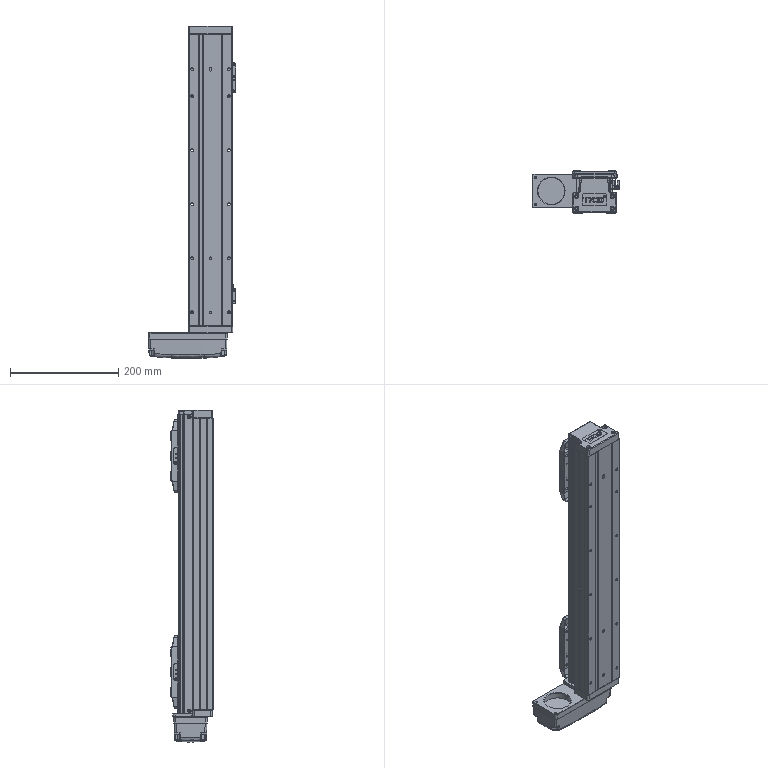Part | 26 solids | 2157 faces | box 161.5 x 78 x 614.5 mm | volume 3064077 mm3 | plane 1049 | cylinder 704 | spline 215 | cone 189 | commonest cylinder face diameters 1 x132 2.5 x64 2 x54 5 x52 5.5 x40 3.3 x32